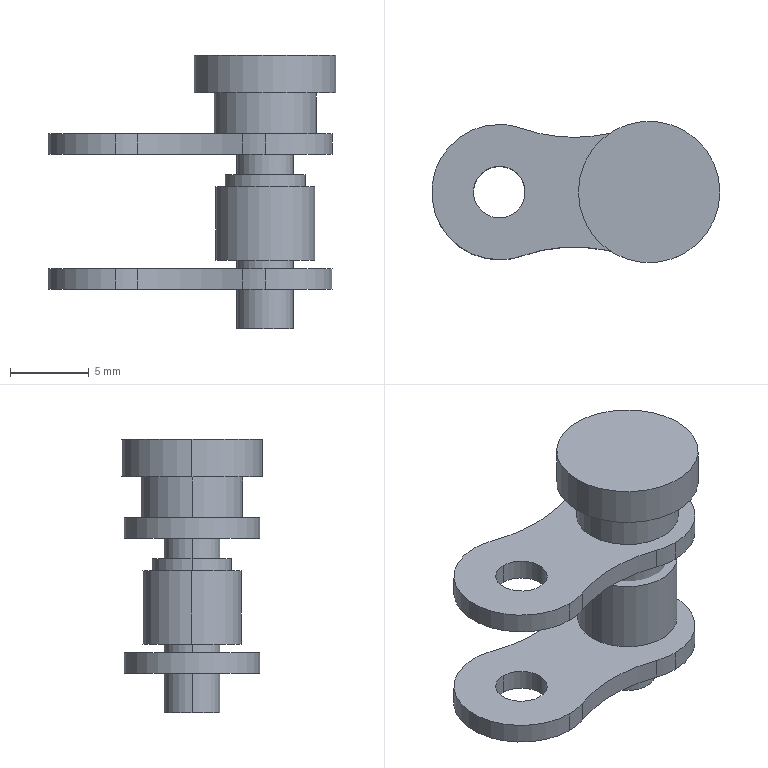Part | STEP file | 06B side guide chain | 4 solids | 50 faces | box 18.325 x 9 x 17.4 mm | volume 854.513 mm3 | cylinder 38 | plane 12 | commonest cylinder face diameters 8.6 x12 3.28 x8 20 x6 3.58 x4 5.08 x2 6.3 x2